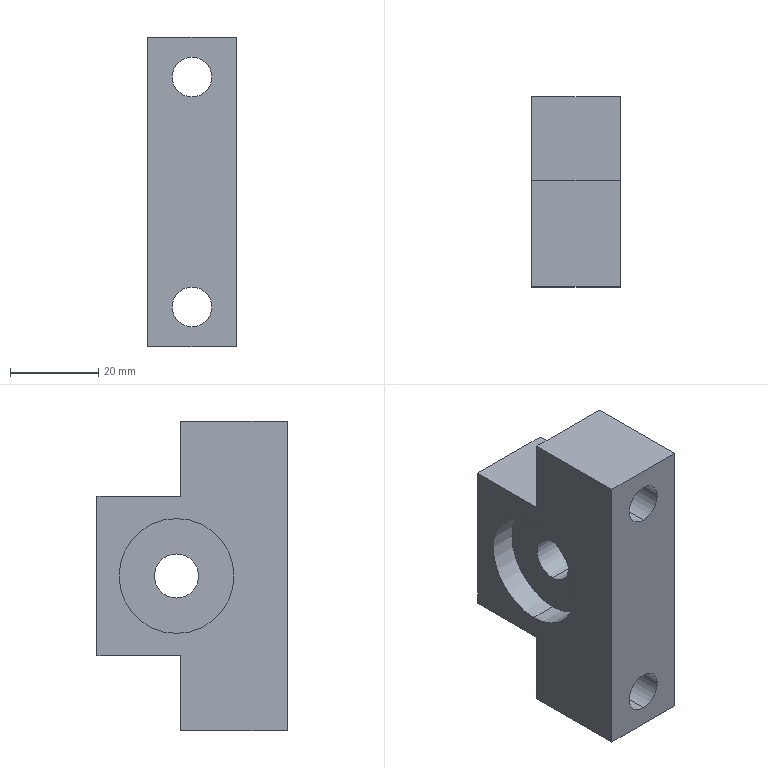Part | SolidWorks | features BaseBody 1 | 1 solid | 22 faces | box 20 x 43 x 70 mm | volume 37227 mm3 | plane 12 | cylinder 10 | commonest cylinder face diameters 9 x4 26 x4 10 x2
STEP:
#1=CARTESIAN_POINT('',(0.,24.,21.5));
#2=VERTEX_POINT('',#1);
#3=CARTESIAN_POINT('',(0.,24.,30.5));
#4=VERTEX_POINT('',#3);
#5=CARTESIAN_POINT('',(0.,24.,26.));
#6=DIRECTION('',(0.,1.,0.));
#7=DIRECTION('',(0.,0.,1.));
#8=AXIS2_PLACEMENT_3D('',#5,#6,#7);
#9=CIRCLE('',#8,4.5);
#10=EDGE_CURVE('',#2,#4,#9,.T.);
#11=ORIENTED_EDGE('',*,*,#10,.F.);
#12=CARTESIAN_POINT('',(0.,24.,26.));
#13=DIRECTION('',(0.,1.,0.));
#14=DIRECTION('',(0.,0.,1.));
#15=AXIS2_PLACEMENT_3D('',#12,#13,#14);
#16=CIRCLE('',#15,4.5);
#17=EDGE_CURVE('',#4,#2,#16,.T.);
#18=ORIENTED_EDGE('',*,*,#17,.F.);
#19=EDGE_LOOP('',(#11,#18));
#20=FACE_BOUND('',#19,.T.);
#21=CARTESIAN_POINT('',(-10.,24.,18.));
#22=VERTEX_POINT('',#21);
#23=CARTESIAN_POINT('',(-10.,24.,35.));
#24=VERTEX_POINT('',#23);
#25=CARTESIAN_POINT('',(-10.,24.,18.));
#26=DIRECTION('',(0.,0.,1.));
#27=VECTOR('',#26,1000.);
#28=LINE('',#25,#27);
#29=EDGE_CURVE('',#22,#24,#28,.T.);
#30=ORIENTED_EDGE('',*,*,#29,.T.);
#31=CARTESIAN_POINT('',(10.,24.,35.));
#32=VERTEX_POINT('',#31);
#33=CARTESIAN_POINT('',(10.,24.,35.));
#34=DIRECTION('',(-1.,0.,0.));
#35=VECTOR('',#34,1000.);
#36=LINE('',#33,#35);
#37=EDGE_CURVE('',#32,#24,#36,.T.);
#38=ORIENTED_EDGE('',*,*,#37,.F.);
#39=CARTESIAN_POINT('',(10.,24.,18.));
#40=VERTEX_POINT('',#39);
#41=CARTESIAN_POINT('',(10.,24.,18.));
#42=DIRECTION('',(0.,0.,1.));
#43=VECTOR('',#42,1000.);
#44=LINE('',#41,#43);
#45=EDGE_CURVE('',#40,#32,#44,.T.);
#46=ORIENTED_EDGE('',*,*,#45,.F.);
#47=CARTESIAN_POINT('',(10.,24.,18.));
#48=DIRECTION('',(-1.,0.,0.));
#49=VECTOR('',#48,1000.);
#50=LINE('',#47,#49);
#51=EDGE_CURVE('',#40,#22,#50,.T.);
#52=ORIENTED_EDGE('',*,*,#51,.T.);
#53=EDGE_LOOP('',(#30,#38,#46,#52));
#54=FACE_OUTER_BOUND('',#53,.T.);
#55=CARTESIAN_POINT('',(10.,24.,18.));
#56=DIRECTION('',(0.,-1.,0.));
#57=DIRECTION('',(0.,0.,-1.));
#58=AXIS2_PLACEMENT_3D('',#55,#56,#57);
#59=PLANE('',#58);
#60=ADVANCED_FACE('',(#20,#54),#59,.F.);
#61=CARTESIAN_POINT('',(-10.,43.,18.));
#62=VERTEX_POINT('',#61);
#63=CARTESIAN_POINT('',(-10.,43.,18.));
#64=DIRECTION('',(0.,-1.,0.));
#65=VECTOR('',#64,1000.);
#66=LINE('',#63,#65);
#67=EDGE_CURVE('',#62,#22,#66,.T.);
#68=ORIENTED_EDGE('',*,*,#67,.T.);
#69=ORIENTED_EDGE('',*,*,#51,.F.);
#70=CARTESIAN_POINT('',(10.,43.,18.));
#71=VERTEX_POINT('',#70);
#72=CARTESIAN_POINT('',(10.,43.,18.));
#73=DIRECTION('',(0.,-1.,0.));
#74=VECTOR('',#73,1000.);
#75=LINE('',#72,#74);
#76=EDGE_CURVE('',#71,#40,#75,.T.);
#77=ORIENTED_EDGE('',*,*,#76,.F.);
#78=CARTESIAN_POINT('',(10.,43.,18.));
#79=DIRECTION('',(-1.,0.,0.));
#80=VECTOR('',#79,1000.);
#81=LINE('',#78,#80);
#82=EDGE_CURVE('',#71,#62,#81,.T.);
#83=ORIENTED_EDGE('',*,*,#82,.T.);
#84=EDGE_LOOP('',(#68,#69,#77,#83));
#85=FACE_OUTER_BOUND('',#84,.T.);
#86=CARTESIAN_POINT('',(10.,43.,18.));
#87=DIRECTION('',(0.,0.,-1.));
#88=DIRECTION('',(-1.,0.,0.));
#89=AXIS2_PLACEMENT_3D('',#86,#87,#88);
#90=PLANE('',#89);
#91=ADVANCED_FACE('',(#85),#90,.F.);
#92=CARTESIAN_POINT('',(-10.,43.,-18.));
#93=VERTEX_POINT('',#92);
#94=CARTESIAN_POINT('',(-10.,43.,-18.));
#95=DIRECTION('',(0.,0.,1.));
#96=VECTOR('',#95,1000.);
#97=LINE('',#94,#96);
#98=EDGE_CURVE('',#93,#62,#97,.T.);
#99=ORIENTED_EDGE('',*,*,#98,.T.);
#100=ORIENTED_EDGE('',*,*,#82,.F.);
#101=CARTESIAN_POINT('',(10.,43.,-18.));
#102=VERTEX_POINT('',#101);
#103=CARTESIAN_POINT('',(10.,43.,-18.));
#104=DIRECTION('',(0.,0.,1.));
#105=VECTOR('',#104,1000.);
#106=LINE('',#103,#105);
#107=EDGE_CURVE('',#102,#71,#106,.T.);
#108=ORIENTED_EDGE('',*,*,#107,.F.);
#109=CARTESIAN_POINT('',(10.,43.,-18.));
#110=DIRECTION('',(-1.,0.,0.));
#111=VECTOR('',#110,1000.);
#112=LINE('',#109,#111);
#113=EDGE_CURVE('',#102,#93,#112,.T.);
#114=ORIENTED_EDGE('',*,*,#113,.T.);
#115=EDGE_LOOP('',(#99,#100,#108,#114));
#116=FACE_OUTER_BOUND('',#115,.T.);
#117=CARTESIAN_POINT('',(10.,43.,-18.));
#118=DIRECTION('',(0.,-1.,0.));
#119=DIRECTION('',(0.,0.,-1.));
#120=AXIS2_PLACEMENT_3D('',#117,#118,#119);
#121=PLANE('',#120);
#122=ADVANCED_FACE('',(#116),#121,.F.);
#123=CARTESIAN_POINT('',(-10.,24.,-18.));
#124=VERTEX_POINT('',#123);
#125=CARTESIAN_POINT('',(-10.,24.,-18.));
#126=DIRECTION('',(0.,1.,0.));
#127=VECTOR('',#126,1000.);
#128=LINE('',#125,#127);
#129=EDGE_CURVE('',#124,#93,#128,.T.);
#130=ORIENTED_EDGE('',*,*,#129,.T.);
#131=ORIENTED_EDGE('',*,*,#113,.F.);
#132=CARTESIAN_POINT('',(10.,24.,-18.));
#133=VERTEX_POINT('',#132);
#134=CARTESIAN_POINT('',(10.,24.,-18.));
#135=DIRECTION('',(0.,1.,0.));
#136=VECTOR('',#135,1000.);
#137=LINE('',#134,#136);
#138=EDGE_CURVE('',#133,#102,#137,.T.);
#139=ORIENTED_EDGE('',*,*,#138,.F.);
#140=CARTESIAN_POINT('',(10.,24.,-18.));
#141=DIRECTION('',(-1.,0.,0.));
#142=VECTOR('',#141,1000.);
#143=LINE('',#140,#142);
#144=EDGE_CURVE('',#133,#124,#143,.T.);
#145=ORIENTED_EDGE('',*,*,#144,.T.);
#146=EDGE_LOOP('',(#130,#131,#139,#145));
#147=FACE_OUTER_BOUND('',#146,.T.);
#148=CARTESIAN_POINT('',(10.,24.,-18.));
#149=DIRECTION('',(0.,0.,1.));
#150=DIRECTION('',(1.,0.,0.));
#151=AXIS2_PLACEMENT_3D('',#148,#149,#150);
#152=PLANE('',#151);
#153=ADVANCED_FACE('',(#147),#152,.F.);
#154=CARTESIAN_POINT('',(0.,24.,-30.5));
#155=VERTEX_POINT('',#154);
#156=CARTESIAN_POINT('',(0.,24.,-21.5));
#157=VERTEX_POINT('',#156);
#158=CARTESIAN_POINT('',(0.,24.,-26.));
#159=DIRECTION('',(0.,-1.,0.));
#160=DIRECTION('',(0.,0.,-1.));
#161=AXIS2_PLACEMENT_3D('',#158,#159,#160);
#162=CIRCLE('',#161,4.5);
#163=EDGE_CURVE('',#155,#157,#162,.T.);
#164=ORIENTED_EDGE('',*,*,#163,.T.);
#165=CARTESIAN_POINT('',(0.,24.,-26.));
#166=DIRECTION('',(0.,-1.,0.));
#167=DIRECTION('',(0.,0.,-1.));
#168=AXIS2_PLACEMENT_3D('',#165,#166,#167);
#169=CIRCLE('',#168,4.5);
#170=EDGE_CURVE('',#157,#155,#169,.T.);
#171=ORIENTED_EDGE('',*,*,#170,.T.);
#172=EDGE_LOOP('',(#164,#171));
#173=FACE_BOUND('',#172,.T.);
#174=CARTESIAN_POINT('',(-10.,24.,-35.));
#175=VERTEX_POINT('',#174);
#176=CARTESIAN_POINT('',(-10.,24.,-35.));
#177=DIRECTION('',(0.,0.,1.));
#178=VECTOR('',#177,1000.);
#179=LINE('',#176,#178);
#180=EDGE_CURVE('',#175,#124,#179,.T.);
#181=ORIENTED_EDGE('',*,*,#180,.T.);
#182=ORIENTED_EDGE('',*,*,#144,.F.);
#183=CARTESIAN_POINT('',(10.,24.,-35.));
#184=VERTEX_POINT('',#183);
#185=CARTESIAN_POINT('',(10.,24.,-35.));
#186=DIRECTION('',(0.,0.,1.));
#187=VECTOR('',#186,1000.);
#188=LINE('',#185,#187);
#189=EDGE_CURVE('',#184,#133,#188,.T.);
#190=ORIENTED_EDGE('',*,*,#189,.F.);
#191=CARTESIAN_POINT('',(10.,24.,-35.));
#192=DIRECTION('',(-1.,0.,0.));
#193=VECTOR('',#192,1000.);
#194=LINE('',#191,#193);
#195=EDGE_CURVE('',#184,#175,#194,.T.);
#196=ORIENTED_EDGE('',*,*,#195,.T.);
#197=EDGE_LOOP('',(#181,#182,#190,#196));
#198=FACE_OUTER_BOUND('',#197,.T.);
#199=CARTESIAN_POINT('',(10.,24.,-35.));
#200=DIRECTION('',(0.,-1.,0.));
#201=DIRECTION('',(0.,0.,-1.));
#202=AXIS2_PLACEMENT_3D('',#199,#200,#201);
#203=PLANE('',#202);
#204=ADVANCED_FACE('',(#173,#198),#203,.F.);
#205=CARTESIAN_POINT('',(-10.,0.,-35.));
#206=VERTEX_POINT('',#205);
#207=CARTESIAN_POINT('',(-10.,0.,-35.));
#208=DIRECTION('',(0.,1.,0.));
#209=VECTOR('',#208,1000.);
#210=LINE('',#207,#209);
#211=EDGE_CURVE('',#206,#175,#210,.T.);
#212=ORIENTED_EDGE('',*,*,#211,.T.);
#213=ORIENTED_EDGE('',*,*,#195,.F.);
#214=CARTESIAN_POINT('',(10.,0.,-35.));
#215=VERTEX_POINT('',#214);
#216=CARTESIAN_POINT('',(10.,0.,-35.));
#217=DIRECTION('',(0.,1.,0.));
#218=VECTOR('',#217,1000.);
#219=LINE('',#216,#218);
#220=EDGE_CURVE('',#215,#184,#219,.T.);
#221=ORIENTED_EDGE('',*,*,#220,.F.);
#222=CARTESIAN_POINT('',(10.,0.,-35.));
#223=DIRECTION('',(-1.,0.,0.));
#224=VECTOR('',#223,1000.);
#225=LINE('',#222,#224);
#226=EDGE_CURVE('',#215,#206,#225,.T.);
#227=ORIENTED_EDGE('',*,*,#226,.T.);
#228=EDGE_LOOP('',(#212,#213,#221,#227));
#229=FACE_OUTER_BOUND('',#228,.T.);
#230=CARTESIAN_POINT('',(10.,0.,-35.));
#231=DIRECTION('',(0.,0.,1.));
#232=DIRECTION('',(1.,0.,0.));
#233=AXIS2_PLACEMENT_3D('',#230,#231,#232);
#234=PLANE('',#233);
#235=ADVANCED_FACE('',(#229),#234,.F.);
#236=CARTESIAN_POINT('',(0.,0.,30.5));
#237=VERTEX_POINT('',#236);
#238=CARTESIAN_POINT('',(0.,0.,21.5));
#239=VERTEX_POINT('',#238);
#240=CARTESIAN_POINT('',(0.,0.,26.));
#241=DIRECTION('',(0.,1.,0.));
#242=DIRECTION('',(0.,0.,1.));
#243=AXIS2_PLACEMENT_3D('',#240,#241,#242);
#244=CIRCLE('',#243,4.5);
#245=EDGE_CURVE('',#237,#239,#244,.T.);
#246=ORIENTED_EDGE('',*,*,#245,.T.);
#247=CARTESIAN_POINT('',(0.,0.,26.));
#248=DIRECTION('',(0.,1.,0.));
#249=DIRECTION('',(0.,0.,1.));
#250=AXIS2_PLACEMENT_3D('',#247,#248,#249);
#251=CIRCLE('',#250,4.5);
#252=EDGE_CURVE('',#239,#237,#251,.T.);
#253=ORIENTED_EDGE('',*,*,#252,.T.);
#254=EDGE_LOOP('',(#246,#253));
#255=FACE_BOUND('',#254,.T.);
#256=CARTESIAN_POINT('',(0.,0.,-21.5));
#257=VERTEX_POINT('',#256);
#258=CARTESIAN_POINT('',(0.,0.,-30.5));
#259=VERTEX_POINT('',#258);
#260=CARTESIAN_POINT('',(0.,0.,-26.));
#261=DIRECTION('',(0.,-1.,0.));
#262=DIRECTION('',(0.,0.,-1.));
#263=AXIS2_PLACEMENT_3D('',#260,#261,#262);
#264=CIRCLE('',#263,4.5);
#265=EDGE_CURVE('',#257,#259,#264,.T.);
#266=ORIENTED_EDGE('',*,*,#265,.F.);
#267=CARTESIAN_POINT('',(0.,0.,-26.));
#268=DIRECTION('',(0.,-1.,0.));
#269=DIRECTION('',(0.,0.,-1.));
#270=AXIS2_PLACEMENT_3D('',#267,#268,#269);
#271=CIRCLE('',#270,4.5);
#272=EDGE_CURVE('',#259,#257,#271,.T.);
#273=ORIENTED_EDGE('',*,*,#272,.F.);
#274=EDGE_LOOP('',(#266,#273));
#275=FACE_BOUND('',#274,.T.);
#276=CARTESIAN_POINT('',(-10.,0.,35.));
#277=VERTEX_POINT('',#276);
#278=CARTESIAN_POINT('',(-10.,0.,35.));
#279=DIRECTION('',(0.,0.,-1.));
#280=VECTOR('',#279,1000.);
#281=LINE('',#278,#280);
#282=EDGE_CURVE('',#277,#206,#281,.T.);
#283=ORIENTED_EDGE('',*,*,#282,.T.);
#284=ORIENTED_EDGE('',*,*,#226,.F.);
#285=CARTESIAN_POINT('',(10.,0.,35.));
#286=VERTEX_POINT('',#285);
#287=CARTESIAN_POINT('',(10.,0.,35.));
#288=DIRECTION('',(0.,0.,-1.));
#289=VECTOR('',#288,1000.);
#290=LINE('',#287,#289);
#291=EDGE_CURVE('',#286,#215,#290,.T.);
#292=ORIENTED_EDGE('',*,*,#291,.F.);
#293=CARTESIAN_POINT('',(10.,0.,35.));
#294=DIRECTION('',(-1.,0.,0.));
#295=VECTOR('',#294,1000.);
#296=LINE('',#293,#295);
#297=EDGE_CURVE('',#286,#277,#296,.T.);
#298=ORIENTED_EDGE('',*,*,#297,.T.);
#299=EDGE_LOOP('',(#283,#284,#292,#298));
#300=FACE_OUTER_BOUND('',#299,.T.);
#301=CARTESIAN_POINT('',(10.,0.,35.));
#302=DIRECTION('',(0.,1.,0.));
#303=DIRECTION('',(0.,0.,1.));
#304=AXIS2_PLACEMENT_3D('',#301,#302,#303);
#305=PLANE('',#304);
#306=ADVANCED_FACE('',(#255,#275,#300),#305,.F.);
#307=CARTESIAN_POINT('',(-10.,24.,35.));
#308=DIRECTION('',(0.,-1.,0.));
#309=VECTOR('',#308,1000.);
#310=LINE('',#307,#309);
#311=EDGE_CURVE('',#24,#277,#310,.T.);
#312=ORIENTED_EDGE('',*,*,#311,.T.);
#313=ORIENTED_EDGE('',*,*,#297,.F.);
#314=CARTESIAN_POINT('',(10.,24.,35.));
#315=DIRECTION('',(0.,-1.,0.));
#316=VECTOR('',#315,1000.);
#317=LINE('',#314,#316);
#318=EDGE_CURVE('',#32,#286,#317,.T.);
#319=ORIENTED_EDGE('',*,*,#318,.F.);
#320=ORIENTED_EDGE('',*,*,#37,.T.);
#321=EDGE_LOOP('',(#312,#313,#319,#320));
#322=FACE_OUTER_BOUND('',#321,.T.);
#323=CARTESIAN_POINT('',(10.,24.,35.));
#324=DIRECTION('',(0.,0.,-1.));
#325=DIRECTION('',(-1.,0.,0.));
#326=AXIS2_PLACEMENT_3D('',#323,#324,#325);
#327=PLANE('',#326);
#328=ADVANCED_FACE('',(#322),#327,.F.);
#329=CARTESIAN_POINT('',(10.,25.,13.));
#330=VERTEX_POINT('',#329);
#331=CARTESIAN_POINT('',(10.,25.,-13.));
#332=VERTEX_POINT('',#331);
#333=CARTESIAN_POINT('',(10.,25.,0.));
#334=DIRECTION('',(1.,0.,0.));
#335=DIRECTION('',(0.,0.,-1.));
#336=AXIS2_PLACEMENT_3D('',#333,#334,#335);
#337=CIRCLE('',#336,13.);
#338=EDGE_CURVE('',#330,#332,#337,.T.);
#339=ORIENTED_EDGE('',*,*,#338,.F.);
#340=CARTESIAN_POINT('',(10.,25.,0.));
#341=DIRECTION('',(1.,0.,0.));
#342=DIRECTION('',(0.,0.,-1.));
#343=AXIS2_PLACEMENT_3D('',#340,#341,#342);
#344=CIRCLE('',#343,13.);
#345=EDGE_CURVE('',#332,#330,#344,.T.);
#346=ORIENTED_EDGE('',*,*,#345,.F.);
#347=EDGE_LOOP('',(#339,#346));
#348=FACE_BOUND('',#347,.T.);
#349=ORIENTED_EDGE('',*,*,#45,.T.);
#350=ORIENTED_EDGE('',*,*,#318,.T.);
#351=ORIENTED_EDGE('',*,*,#291,.T.);
#352=ORIENTED_EDGE('',*,*,#220,.T.);
#353=ORIENTED_EDGE('',*,*,#189,.T.);
#354=ORIENTED_EDGE('',*,*,#138,.T.);
#355=ORIENTED_EDGE('',*,*,#107,.T.);
#356=ORIENTED_EDGE('',*,*,#76,.T.);
#357=EDGE_LOOP('',(#349,#350,#351,#352,#353,#354,#355,#356));
#358=FACE_OUTER_BOUND('',#357,.T.);
#359=CARTESIAN_POINT('',(10.,0.,0.));
#360=DIRECTION('',(1.,0.,0.));
#361=DIRECTION('',(0.,0.,-1.));
#362=AXIS2_PLACEMENT_3D('',#359,#360,#361);
#363=PLANE('',#362);
#364=ADVANCED_FACE('',(#348,#358),#363,.T.);
#365=CARTESIAN_POINT('',(4.,25.,13.));
#366=VERTEX_POINT('',#365);
#367=CARTESIAN_POINT('',(4.,25.,13.));
#368=DIRECTION('',(1.,0.,0.));
#369=VECTOR('',#368,1000.);
#370=LINE('',#367,#369);
#371=EDGE_CURVE('',#366,#330,#370,.T.);
#372=ORIENTED_EDGE('',*,*,#371,.F.);
#373=CARTESIAN_POINT('',(4.,25.,-13.));
#374=VERTEX_POINT('',#373);
#375=CARTESIAN_POINT('',(4.,25.,0.));
#376=DIRECTION('',(1.,0.,0.));
#377=DIRECTION('',(0.,0.,-1.));
#378=AXIS2_PLACEMENT_3D('',#375,#376,#377);
#379=CIRCLE('',#378,13.);
#380=EDGE_CURVE('',#374,#366,#379,.T.);
#381=ORIENTED_EDGE('',*,*,#380,.F.);
#382=CARTESIAN_POINT('',(4.,25.,-13.));
#383=DIRECTION('',(1.,0.,0.));
#384=VECTOR('',#383,1000.);
#385=LINE('',#382,#384);
#386=EDGE_CURVE('',#374,#332,#385,.T.);
#387=ORIENTED_EDGE('',*,*,#386,.T.);
#388=ORIENTED_EDGE('',*,*,#345,.T.);
#389=EDGE_LOOP('',(#372,#381,#387,#388));
#390=FACE_OUTER_BOUND('',#389,.T.);
#391=CARTESIAN_POINT('',(10.,25.,0.));
#392=DIRECTION('',(1.,0.,0.));
#393=DIRECTION('',(0.,-1.,0.));
#394=AXIS2_PLACEMENT_3D('',#391,#392,#393);
#395=CYLINDRICAL_SURFACE('',#394,13.);
#396=ADVANCED_FACE('',(#390),#395,.F.);
#397=ORIENTED_EDGE('',*,*,#371,.T.);
#398=ORIENTED_EDGE('',*,*,#338,.T.);
#399=ORIENTED_EDGE('',*,*,#386,.F.);
#400=CARTESIAN_POINT('',(4.,25.,0.));
#401=DIRECTION('',(1.,0.,0.));
#402=DIRECTION('',(0.,0.,-1.));
#403=AXIS2_PLACEMENT_3D('',#400,#401,#402);
#404=CIRCLE('',#403,13.);
#405=EDGE_CURVE('',#366,#374,#404,.T.);
#406=ORIENTED_EDGE('',*,*,#405,.F.);
#407=EDGE_LOOP('',(#397,#398,#399,#406));
#408=FACE_OUTER_BOUND('',#407,.T.);
#409=CARTESIAN_POINT('',(10.,25.,0.));
#410=DIRECTION('',(1.,0.,0.));
#411=DIRECTION('',(0.,1.,0.));
#412=AXIS2_PLACEMENT_3D('',#409,#410,#411);
#413=CYLINDRICAL_SURFACE('',#412,13.);
#414=ADVANCED_FACE('',(#408),#413,.F.);
#415=ORIENTED_EDGE('',*,*,#380,.T.);
#416=ORIENTED_EDGE('',*,*,#405,.T.);
#417=EDGE_LOOP('',(#415,#416));
#418=FACE_OUTER_BOUND('',#417,.T.);
#419=CARTESIAN_POINT('',(4.,25.,5.));
#420=VERTEX_POINT('',#419);
#421=CARTESIAN_POINT('',(4.,25.,-5.));
#422=VERTEX_POINT('',#421);
#423=CARTESIAN_POINT('',(4.,25.,0.));
#424=DIRECTION('',(1.,0.,0.));
#425=DIRECTION('',(0.,0.,-1.));
#426=AXIS2_PLACEMENT_3D('',#423,#424,#425);
#427=CIRCLE('',#426,5.);
#428=EDGE_CURVE('',#420,#422,#427,.T.);
#429=ORIENTED_EDGE('',*,*,#428,.F.);
#430=CARTESIAN_POINT('',(4.,25.,0.));
#431=DIRECTION('',(1.,0.,0.));
#432=DIRECTION('',(0.,0.,-1.));
#433=AXIS2_PLACEMENT_3D('',#430,#431,#432);
#434=CIRCLE('',#433,5.);
#435=EDGE_CURVE('',#422,#420,#434,.T.);
#436=ORIENTED_EDGE('',*,*,#435,.F.);
#437=EDGE_LOOP('',(#429,#436));
#438=FACE_BOUND('',#437,.T.);
#439=CARTESIAN_POINT('',(4.,30.,0.));
#440=DIRECTION('',(1.,0.,0.));
#441=DIRECTION('',(0.,0.,-1.));
#442=AXIS2_PLACEMENT_3D('',#439,#440,#441);
#443=PLANE('',#442);
#444=ADVANCED_FACE('',(#418,#438),#443,.T.);
#445=CARTESIAN_POINT('',(-4.,25.,5.));
#446=VERTEX_POINT('',#445);
#447=CARTESIAN_POINT('',(-4.,25.,5.));
#448=DIRECTION('',(1.,0.,0.));
#449=VECTOR('',#448,1000.);
#450=LINE('',#447,#449);
#451=EDGE_CURVE('',#446,#420,#450,.T.);
#452=ORIENTED_EDGE('',*,*,#451,.F.);
#453=CARTESIAN_POINT('',(-4.,25.,-5.));
#454=VERTEX_POINT('',#453);
#455=CARTESIAN_POINT('',(-4.,25.,0.));
#456=DIRECTION('',(1.,0.,0.));
#457=DIRECTION('',(0.,0.,-1.));
#458=AXIS2_PLACEMENT_3D('',#455,#456,#457);
#459=CIRCLE('',#458,5.);
#460=EDGE_CURVE('',#454,#446,#459,.T.);
#461=ORIENTED_EDGE('',*,*,#460,.F.);
#462=CARTESIAN_POINT('',(-4.,25.,-5.));
#463=DIRECTION('',(1.,0.,0.));
#464=VECTOR('',#463,1000.);
#465=LINE('',#462,#464);
#466=EDGE_CURVE('',#454,#422,#465,.T.);
#467=ORIENTED_EDGE('',*,*,#466,.T.);
#468=ORIENTED_EDGE('',*,*,#435,.T.);
#469=EDGE_LOOP('',(#452,#461,#467,#468));
#470=FACE_OUTER_BOUND('',#469,.T.);
#471=CARTESIAN_POINT('',(10.,25.,0.));
#472=DIRECTION('',(1.,0.,0.));
#473=DIRECTION('',(0.,-1.,0.));
#474=AXIS2_PLACEMENT_3D('',#471,#472,#473);
#475=CYLINDRICAL_SURFACE('',#474,5.);
#476=ADVANCED_FACE('',(#470),#475,.F.);
#477=ORIENTED_EDGE('',*,*,#451,.T.);
#478=ORIENTED_EDGE('',*,*,#428,.T.);
#479=ORIENTED_EDGE('',*,*,#466,.F.);
#480=CARTESIAN_POINT('',(-4.,25.,0.));
#481=DIRECTION('',(1.,0.,0.));
#482=DIRECTION('',(0.,0.,-1.));
#483=AXIS2_PLACEMENT_3D('',#480,#481,#482);
#484=CIRCLE('',#483,5.);
#485=EDGE_CURVE('',#446,#454,#484,.T.);
#486=ORIENTED_EDGE('',*,*,#485,.F.);
#487=EDGE_LOOP('',(#477,#478,#479,#486));
#488=FACE_OUTER_BOUND('',#487,.T.);
#489=CARTESIAN_POINT('',(10.,25.,0.));
#490=DIRECTION('',(1.,0.,0.));
#491=DIRECTION('',(0.,1.,0.));
#492=AXIS2_PLACEMENT_3D('',#489,#490,#491);
#493=CYLINDRICAL_SURFACE('',#492,5.);
#494=ADVANCED_FACE('',(#488),#493,.F.);
#495=ORIENTED_EDGE('',*,*,#460,.T.);
#496=ORIENTED_EDGE('',*,*,#485,.T.);
#497=EDGE_LOOP('',(#495,#496));
#498=FACE_BOUND('',#497,.T.);
#499=CARTESIAN_POINT('',(-4.,25.,13.));
#500=VERTEX_POINT('',#499);
#501=CARTESIAN_POINT('',(-4.,25.,-13.));
#502=VERTEX_POINT('',#501);
#503=CARTESIAN_POINT('',(-4.,25.,0.));
#504=DIRECTION('',(1.,0.,0.));
#505=DIRECTION('',(0.,0.,-1.));
#506=AXIS2_PLACEMENT_3D('',#503,#504,#505);
#507=CIRCLE('',#506,13.);
#508=EDGE_CURVE('',#500,#502,#507,.T.);
#509=ORIENTED_EDGE('',*,*,#508,.F.);
#510=CARTESIAN_POINT('',(-4.,25.,0.));
#511=DIRECTION('',(1.,0.,0.));
#512=DIRECTION('',(0.,0.,-1.));
#513=AXIS2_PLACEMENT_3D('',#510,#511,#512);
#514=CIRCLE('',#513,13.);
#515=EDGE_CURVE('',#502,#500,#514,.T.);
#516=ORIENTED_EDGE('',*,*,#515,.F.);
#517=EDGE_LOOP('',(#509,#516));
#518=FACE_OUTER_BOUND('',#517,.T.);
#519=CARTESIAN_POINT('',(-4.,38.,0.));
#520=DIRECTION('',(-1.,0.,0.));
#521=DIRECTION('',(0.,0.,1.));
#522=AXIS2_PLACEMENT_3D('',#519,#520,#521);
#523=PLANE('',#522);
#524=ADVANCED_FACE('',(#498,#518),#523,.T.);
#525=CARTESIAN_POINT('',(-10.,25.,13.));
#526=VERTEX_POINT('',#525);
#527=CARTESIAN_POINT('',(-10.,25.,13.));
#528=DIRECTION('',(1.,0.,0.));
#529=VECTOR('',#528,1000.);
#530=LINE('',#527,#529);
#531=EDGE_CURVE('',#526,#500,#530,.T.);
#532=ORIENTED_EDGE('',*,*,#531,.F.);
#533=CARTESIAN_POINT('',(-10.,25.,-13.));
#534=VERTEX_POINT('',#533);
#535=CARTESIAN_POINT('',(-10.,25.,0.));
#536=DIRECTION('',(1.,0.,0.));
#537=DIRECTION('',(0.,0.,-1.));
#538=AXIS2_PLACEMENT_3D('',#535,#536,#537);
#539=CIRCLE('',#538,13.);
#540=EDGE_CURVE('',#534,#526,#539,.T.);
#541=ORIENTED_EDGE('',*,*,#540,.F.);
#542=CARTESIAN_POINT('',(-10.,25.,-13.));
#543=DIRECTION('',(1.,0.,0.));
#544=VECTOR('',#543,1000.);
#545=LINE('',#542,#544);
#546=EDGE_CURVE('',#534,#502,#545,.T.);
#547=ORIENTED_EDGE('',*,*,#546,.T.);
#548=ORIENTED_EDGE('',*,*,#515,.T.);
#549=EDGE_LOOP('',(#532,#541,#547,#548));
#550=FACE_OUTER_BOUND('',#549,.T.);
#551=CARTESIAN_POINT('',(10.,25.,0.));
#552=DIRECTION('',(1.,0.,0.));
#553=DIRECTION('',(0.,-1.,0.));
#554=AXIS2_PLACEMENT_3D('',#551,#552,#553);
#555=CYLINDRICAL_SURFACE('',#554,13.);
#556=ADVANCED_FACE('',(#550),#555,.F.);
#557=ORIENTED_EDGE('',*,*,#531,.T.);
#558=ORIENTED_EDGE('',*,*,#508,.T.);
#559=ORIENTED_EDGE('',*,*,#546,.F.);
#560=CARTESIAN_POINT('',(-10.,25.,0.));
#561=DIRECTION('',(1.,0.,0.));
#562=DIRECTION('',(0.,0.,-1.));
#563=AXIS2_PLACEMENT_3D('',#560,#561,#562);
#564=CIRCLE('',#563,13.);
#565=EDGE_CURVE('',#526,#534,#564,.T.);
#566=ORIENTED_EDGE('',*,*,#565,.F.);
#567=EDGE_LOOP('',(#557,#558,#559,#566));
#568=FACE_OUTER_BOUND('',#567,.T.);
#569=CARTESIAN_POINT('',(10.,25.,0.));
#570=DIRECTION('',(1.,0.,0.));
#571=DIRECTION('',(0.,1.,0.));
#572=AXIS2_PLACEMENT_3D('',#569,#570,#571);
#573=CYLINDRICAL_SURFACE('',#572,13.);
#574=ADVANCED_FACE('',(#568),#573,.F.);
#575=ORIENTED_EDGE('',*,*,#540,.T.);
#576=ORIENTED_EDGE('',*,*,#565,.T.);
#577=EDGE_LOOP('',(#575,#576));
#578=FACE_BOUND('',#577,.T.);
#579=ORIENTED_EDGE('',*,*,#29,.F.);
#580=ORIENTED_EDGE('',*,*,#67,.F.);
#581=ORIENTED_EDGE('',*,*,#98,.F.);
#582=ORIENTED_EDGE('',*,*,#129,.F.);
#583=ORIENTED_EDGE('',*,*,#180,.F.);
#584=ORIENTED_EDGE('',*,*,#211,.F.);
#585=ORIENTED_EDGE('',*,*,#282,.F.);
#586=ORIENTED_EDGE('',*,*,#311,.F.);
#587=EDGE_LOOP('',(#579,#580,#581,#582,#583,#584,#585,#586));
#588=FACE_OUTER_BOUND('',#587,.T.);
#589=CARTESIAN_POINT('',(-10.,0.,0.));
#590=DIRECTION('',(1.,0.,0.));
#591=DIRECTION('',(0.,0.,-1.));
#592=AXIS2_PLACEMENT_3D('',#589,#590,#591);
#593=PLANE('',#592);
#594=ADVANCED_FACE('',(#578,#588),#593,.F.);
#595=CARTESIAN_POINT('',(0.,24.,-21.5));
#596=DIRECTION('',(0.,-1.,0.));
#597=VECTOR('',#596,1000.);
#598=LINE('',#595,#597);
#599=EDGE_CURVE('',#157,#257,#598,.T.);
#600=ORIENTED_EDGE('',*,*,#599,.F.);
#601=ORIENTED_EDGE('',*,*,#163,.F.);
#602=CARTESIAN_POINT('',(0.,24.,-30.5));
#603=DIRECTION('',(0.,-1.,0.));
#604=VECTOR('',#603,1000.);
#605=LINE('',#602,#604);
#606=EDGE_CURVE('',#155,#259,#605,.T.);
#607=ORIENTED_EDGE('',*,*,#606,.T.);
#608=ORIENTED_EDGE('',*,*,#272,.T.);
#609=EDGE_LOOP('',(#600,#601,#607,#608));
#610=FACE_OUTER_BOUND('',#609,.T.);
#611=CARTESIAN_POINT('',(0.,0.,-26.));
#612=DIRECTION('',(0.,-1.,0.));
#613=DIRECTION('',(-1.,0.,0.));
#614=AXIS2_PLACEMENT_3D('',#611,#612,#613);
#615=CYLINDRICAL_SURFACE('',#614,4.5);
#616=ADVANCED_FACE('',(#610),#615,.F.);
#617=ORIENTED_EDGE('',*,*,#599,.T.);
#618=ORIENTED_EDGE('',*,*,#265,.T.);
#619=ORIENTED_EDGE('',*,*,#606,.F.);
#620=ORIENTED_EDGE('',*,*,#170,.F.);
#621=EDGE_LOOP('',(#617,#618,#619,#620));
#622=FACE_OUTER_BOUND('',#621,.T.);
#623=CARTESIAN_POINT('',(0.,0.,-26.));
#624=DIRECTION('',(0.,-1.,0.));
#625=DIRECTION('',(1.,0.,0.));
#626=AXIS2_PLACEMENT_3D('',#623,#624,#625);
#627=CYLINDRICAL_SURFACE('',#626,4.5);
#628=ADVANCED_FACE('',(#622),#627,.F.);
#629=CARTESIAN_POINT('',(0.,0.,21.5));
#630=DIRECTION('',(0.,1.,0.));
#631=VECTOR('',#630,1000.);
#632=LINE('',#629,#631);
#633=EDGE_CURVE('',#239,#2,#632,.T.);
#634=ORIENTED_EDGE('',*,*,#633,.T.);
#635=ORIENTED_EDGE('',*,*,#10,.T.);
#636=CARTESIAN_POINT('',(0.,0.,30.5));
#637=DIRECTION('',(0.,1.,0.));
#638=VECTOR('',#637,1000.);
#639=LINE('',#636,#638);
#640=EDGE_CURVE('',#237,#4,#639,.T.);
#641=ORIENTED_EDGE('',*,*,#640,.F.);
#642=ORIENTED_EDGE('',*,*,#252,.F.);
#643=EDGE_LOOP('',(#634,#635,#641,#642));
#644=FACE_OUTER_BOUND('',#643,.T.);
#645=CARTESIAN_POINT('',(0.,24.,26.));
#646=DIRECTION('',(0.,1.,0.));
#647=DIRECTION('',(1.,0.,0.));
#648=AXIS2_PLACEMENT_3D('',#645,#646,#647);
#649=CYLINDRICAL_SURFACE('',#648,4.5);
#650=ADVANCED_FACE('',(#644),#649,.F.);
#651=ORIENTED_EDGE('',*,*,#633,.F.);
#652=ORIENTED_EDGE('',*,*,#245,.F.);
#653=ORIENTED_EDGE('',*,*,#640,.T.);
#654=ORIENTED_EDGE('',*,*,#17,.T.);
#655=EDGE_LOOP('',(#651,#652,#653,#654));
#656=FACE_OUTER_BOUND('',#655,.T.);
#657=CARTESIAN_POINT('',(0.,24.,26.));
#658=DIRECTION('',(0.,1.,0.));
#659=DIRECTION('',(-1.,0.,0.));
#660=AXIS2_PLACEMENT_3D('',#657,#658,#659);
#661=CYLINDRICAL_SURFACE('',#660,4.5);
#662=ADVANCED_FACE('',(#656),#661,.F.);
#663=CLOSED_SHELL('',(#60,#91,#122,#153,#204,#235,#306,#328,#364,#396,#414,#444,#476,#494,#524,#556,#574,#594,#616,#628,#650,#662));
#664=MANIFOLD_SOLID_BREP('',#663);
#665=CARTESIAN_POINT('',(0.,0.,0.));
#666=DIRECTION('',(0.,0.,1.));
#667=DIRECTION('',(1.,0.,0.));
#668=AXIS2_PLACEMENT_3D('',#665,#666,#667);
#669=(LENGTH_UNIT()NAMED_UNIT(*)SI_UNIT(.MILLI.,.METRE.));
#670=UNCERTAINTY_MEASURE_WITH_UNIT(LENGTH_MEASURE(0.00001),#669,'','');
#671=(NAMED_UNIT(*)PLANE_ANGLE_UNIT()SI_UNIT($,.RADIAN.));
#672=(NAMED_UNIT(*)SI_UNIT($,.STERADIAN.)SOLID_ANGLE_UNIT());
#673=(GEOMETRIC_REPRESENTATION_CONTEXT(3)GLOBAL_UNCERTAINTY_ASSIGNED_CONTEXT((#670))GLOBAL_UNIT_ASSIGNED_CONTEXT((#669,#671,#672))REPRESENTATION_CONTEXT('',''));
#674=ADVANCED_BREP_SHAPE_REPRESENTATION('',(#664,#668),#673);